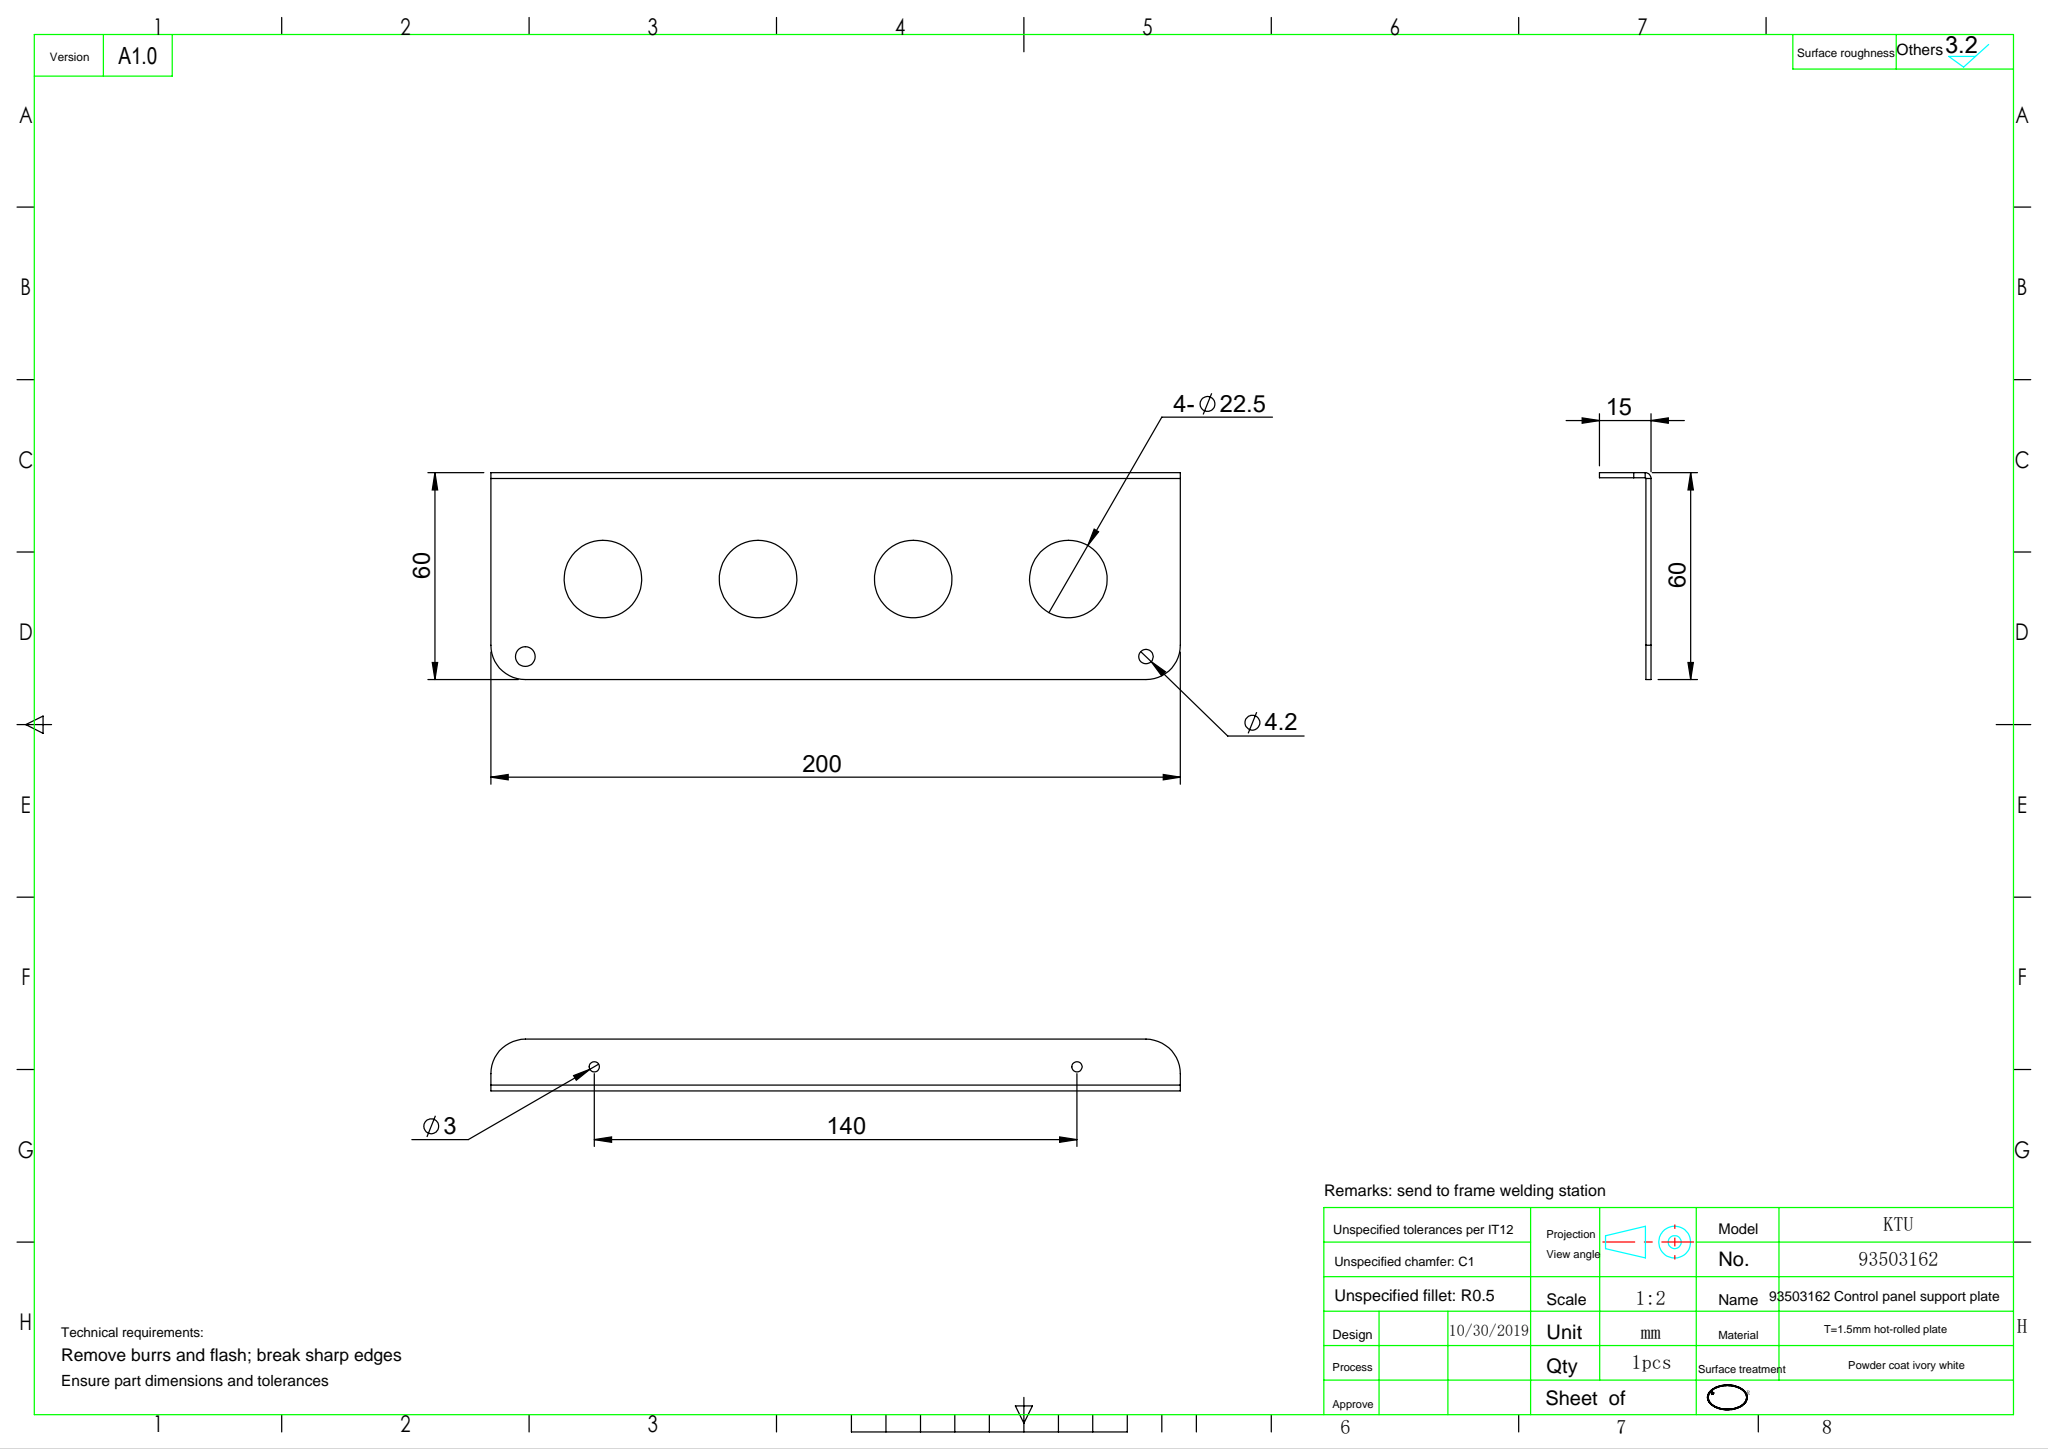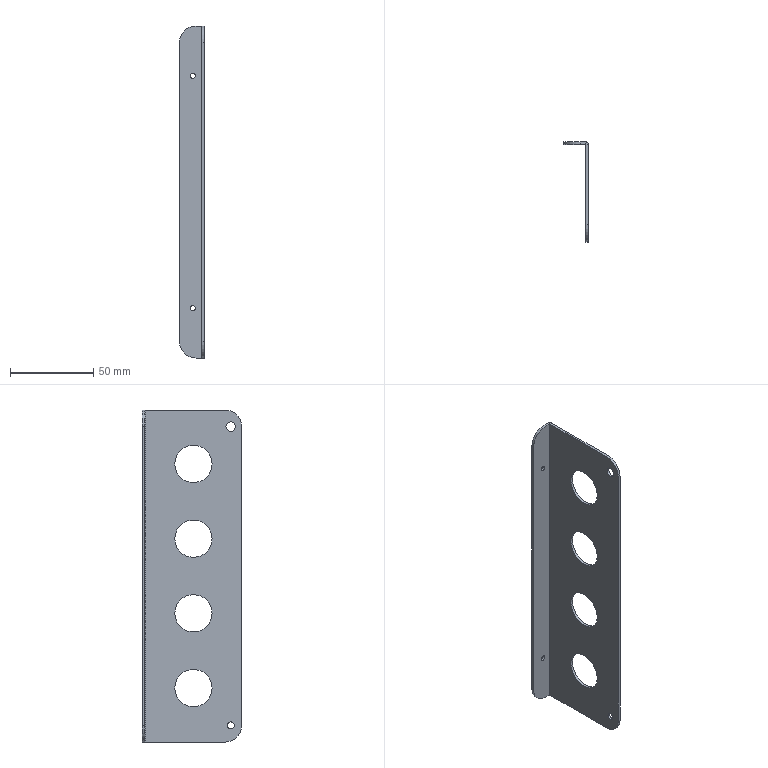Part | SolidWorks | features ICE 3, Fillet 1, FlatPattern 1, SMBaseFlange 1, SheetMetal 1 | 1 solid | 34 faces | box 15 x 60 x 200 mm | volume 19332 mm3 | cylinder 22 | plane 12 | commonest cylinder face diameters 22.5 x8 3 x4 20 x4 4.2 x2 5.744 x2 0.4 x1